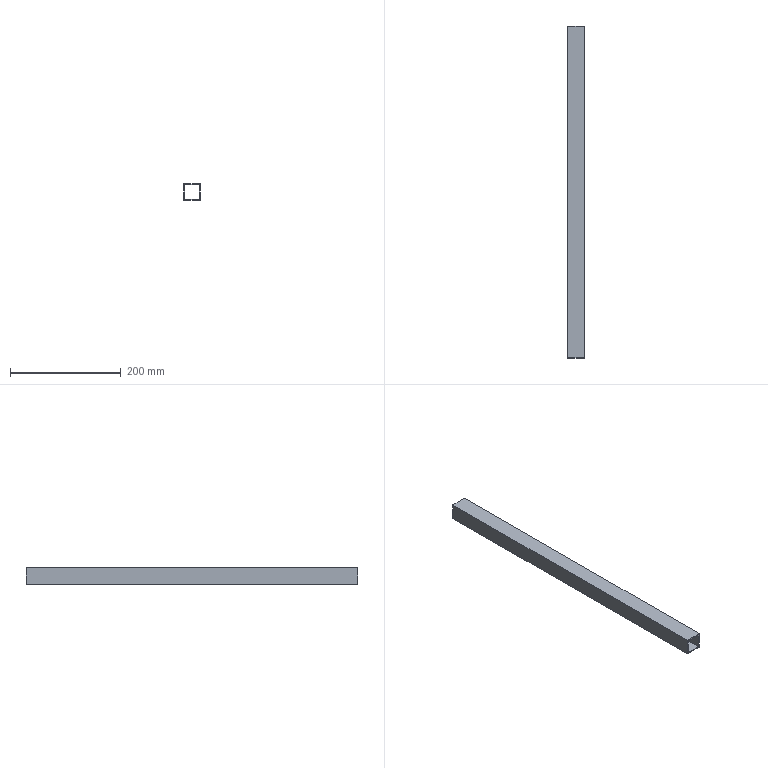Part | NX | features solid 2 | 1 solid | 10 faces | box 30 x 600 x 30 mm | volume 134400 mm3 | plane 10
STEP:
#1=CARTESIAN_POINT('',(-135.,-330.,-30.));
#2=VERTEX_POINT('',#1);
#3=CARTESIAN_POINT('',(-105.,-330.,-30.));
#4=VERTEX_POINT('',#3);
#5=CARTESIAN_POINT('',(-320.,-330.,-30.));
#6=DIRECTION('',(1.,0.,0.));
#7=VECTOR('',#6,1000.);
#8=LINE('',#5,#7);
#9=EDGE_CURVE('',#2,#4,#8,.T.);
#10=ORIENTED_EDGE('',*,*,#9,.T.);
#11=CARTESIAN_POINT('',(-105.,-330.,0.));
#12=VERTEX_POINT('',#11);
#13=CARTESIAN_POINT('',(-105.,-330.,0.));
#14=DIRECTION('',(0.,0.,-1.));
#15=VECTOR('',#14,1000.);
#16=LINE('',#13,#15);
#17=EDGE_CURVE('',#12,#4,#16,.T.);
#18=ORIENTED_EDGE('',*,*,#17,.F.);
#19=CARTESIAN_POINT('',(-135.,-330.,0.));
#20=VERTEX_POINT('',#19);
#21=CARTESIAN_POINT('',(-320.,-330.,0.));
#22=DIRECTION('',(1.,0.,0.));
#23=VECTOR('',#22,1000.);
#24=LINE('',#21,#23);
#25=EDGE_CURVE('',#20,#12,#24,.T.);
#26=ORIENTED_EDGE('',*,*,#25,.F.);
#27=CARTESIAN_POINT('',(-135.,-330.,0.));
#28=DIRECTION('',(0.,0.,-1.));
#29=VECTOR('',#28,1000.);
#30=LINE('',#27,#29);
#31=EDGE_CURVE('',#20,#2,#30,.T.);
#32=ORIENTED_EDGE('',*,*,#31,.T.);
#33=EDGE_LOOP('',(#10,#18,#26,#32));
#34=FACE_BOUND('',#33,.T.);
#35=CARTESIAN_POINT('',(-133.,-330.,-28.));
#36=VERTEX_POINT('',#35);
#37=CARTESIAN_POINT('',(-107.,-330.,-28.));
#38=VERTEX_POINT('',#37);
#39=CARTESIAN_POINT('',(-320.,-330.,-28.));
#40=DIRECTION('',(1.,0.,0.));
#41=VECTOR('',#40,1000.);
#42=LINE('',#39,#41);
#43=EDGE_CURVE('',#36,#38,#42,.T.);
#44=ORIENTED_EDGE('',*,*,#43,.F.);
#45=CARTESIAN_POINT('',(-133.,-330.,-2.));
#46=VERTEX_POINT('',#45);
#47=CARTESIAN_POINT('',(-133.,-330.,0.));
#48=DIRECTION('',(0.,0.,-1.));
#49=VECTOR('',#48,1000.);
#50=LINE('',#47,#49);
#51=EDGE_CURVE('',#46,#36,#50,.T.);
#52=ORIENTED_EDGE('',*,*,#51,.F.);
#53=CARTESIAN_POINT('',(-107.,-330.,-2.));
#54=VERTEX_POINT('',#53);
#55=CARTESIAN_POINT('',(-320.,-330.,-2.));
#56=DIRECTION('',(1.,0.,0.));
#57=VECTOR('',#56,1000.);
#58=LINE('',#55,#57);
#59=EDGE_CURVE('',#46,#54,#58,.T.);
#60=ORIENTED_EDGE('',*,*,#59,.T.);
#61=CARTESIAN_POINT('',(-107.,-330.,0.));
#62=DIRECTION('',(0.,0.,-1.));
#63=VECTOR('',#62,1000.);
#64=LINE('',#61,#63);
#65=EDGE_CURVE('',#54,#38,#64,.T.);
#66=ORIENTED_EDGE('',*,*,#65,.T.);
#67=EDGE_LOOP('',(#44,#52,#60,#66));
#68=FACE_BOUND('',#67,.T.);
#69=CARTESIAN_POINT('',(-320.,-330.,0.));
#70=DIRECTION('',(0.,1.,0.));
#71=DIRECTION('',(0.,0.,1.));
#72=AXIS2_PLACEMENT_3D('',#69,#70,#71);
#73=PLANE('',#72);
#74=ADVANCED_FACE('',(#34,#68),#73,.F.);
#75=CARTESIAN_POINT('',(-135.,270.,0.));
#76=VERTEX_POINT('',#75);
#77=CARTESIAN_POINT('',(-135.,-330.,0.));
#78=DIRECTION('',(0.,1.,0.));
#79=VECTOR('',#78,1000.);
#80=LINE('',#77,#79);
#81=EDGE_CURVE('',#20,#76,#80,.T.);
#82=ORIENTED_EDGE('',*,*,#81,.T.);
#83=CARTESIAN_POINT('',(-135.,270.,-30.));
#84=VERTEX_POINT('',#83);
#85=CARTESIAN_POINT('',(-135.,270.,0.));
#86=DIRECTION('',(0.,0.,1.));
#87=VECTOR('',#86,1000.);
#88=LINE('',#85,#87);
#89=EDGE_CURVE('',#84,#76,#88,.T.);
#90=ORIENTED_EDGE('',*,*,#89,.F.);
#91=CARTESIAN_POINT('',(-135.,-330.,-30.));
#92=DIRECTION('',(0.,1.,0.));
#93=VECTOR('',#92,1000.);
#94=LINE('',#91,#93);
#95=EDGE_CURVE('',#2,#84,#94,.T.);
#96=ORIENTED_EDGE('',*,*,#95,.F.);
#97=ORIENTED_EDGE('',*,*,#31,.F.);
#98=EDGE_LOOP('',(#82,#90,#96,#97));
#99=FACE_BOUND('',#98,.T.);
#100=CARTESIAN_POINT('',(-135.,-330.,0.));
#101=DIRECTION('',(-1.,0.,0.));
#102=DIRECTION('',(0.,0.,1.));
#103=AXIS2_PLACEMENT_3D('',#100,#101,#102);
#104=PLANE('',#103);
#105=ADVANCED_FACE('',(#99),#104,.T.);
#106=CARTESIAN_POINT('',(-105.,270.,-30.));
#107=VERTEX_POINT('',#106);
#108=CARTESIAN_POINT('',(-105.,-330.,-30.));
#109=DIRECTION('',(0.,1.,0.));
#110=VECTOR('',#109,1000.);
#111=LINE('',#108,#110);
#112=EDGE_CURVE('',#4,#107,#111,.T.);
#113=ORIENTED_EDGE('',*,*,#112,.T.);
#114=CARTESIAN_POINT('',(-105.,270.,0.));
#115=VERTEX_POINT('',#114);
#116=CARTESIAN_POINT('',(-105.,270.,0.));
#117=DIRECTION('',(0.,0.,1.));
#118=VECTOR('',#117,1000.);
#119=LINE('',#116,#118);
#120=EDGE_CURVE('',#107,#115,#119,.T.);
#121=ORIENTED_EDGE('',*,*,#120,.T.);
#122=CARTESIAN_POINT('',(-105.,-330.,0.));
#123=DIRECTION('',(0.,1.,0.));
#124=VECTOR('',#123,1000.);
#125=LINE('',#122,#124);
#126=EDGE_CURVE('',#12,#115,#125,.T.);
#127=ORIENTED_EDGE('',*,*,#126,.F.);
#128=ORIENTED_EDGE('',*,*,#17,.T.);
#129=EDGE_LOOP('',(#113,#121,#127,#128));
#130=FACE_BOUND('',#129,.T.);
#131=CARTESIAN_POINT('',(-105.,-330.,0.));
#132=DIRECTION('',(-1.,0.,0.));
#133=DIRECTION('',(0.,0.,1.));
#134=AXIS2_PLACEMENT_3D('',#131,#132,#133);
#135=PLANE('',#134);
#136=ADVANCED_FACE('',(#130),#135,.F.);
#137=ORIENTED_EDGE('',*,*,#126,.T.);
#138=CARTESIAN_POINT('',(-248.75,270.,0.));
#139=DIRECTION('',(1.,0.,0.));
#140=VECTOR('',#139,1000.);
#141=LINE('',#138,#140);
#142=EDGE_CURVE('',#76,#115,#141,.T.);
#143=ORIENTED_EDGE('',*,*,#142,.F.);
#144=ORIENTED_EDGE('',*,*,#81,.F.);
#145=ORIENTED_EDGE('',*,*,#25,.T.);
#146=EDGE_LOOP('',(#137,#143,#144,#145));
#147=FACE_BOUND('',#146,.T.);
#148=CARTESIAN_POINT('',(-248.75,-180.,0.));
#149=DIRECTION('',(0.,0.,1.));
#150=DIRECTION('',(1.,0.,0.));
#151=AXIS2_PLACEMENT_3D('',#148,#149,#150);
#152=PLANE('',#151);
#153=ADVANCED_FACE('',(#147),#152,.T.);
#154=ORIENTED_EDGE('',*,*,#95,.T.);
#155=CARTESIAN_POINT('',(-248.75,270.,-30.));
#156=DIRECTION('',(1.,0.,0.));
#157=VECTOR('',#156,1000.);
#158=LINE('',#155,#157);
#159=EDGE_CURVE('',#84,#107,#158,.T.);
#160=ORIENTED_EDGE('',*,*,#159,.T.);
#161=ORIENTED_EDGE('',*,*,#112,.F.);
#162=ORIENTED_EDGE('',*,*,#9,.F.);
#163=EDGE_LOOP('',(#154,#160,#161,#162));
#164=FACE_BOUND('',#163,.T.);
#165=CARTESIAN_POINT('',(-248.75,-180.,-30.));
#166=DIRECTION('',(0.,0.,1.));
#167=DIRECTION('',(1.,0.,0.));
#168=AXIS2_PLACEMENT_3D('',#165,#166,#167);
#169=PLANE('',#168);
#170=ADVANCED_FACE('',(#164),#169,.F.);
#171=CARTESIAN_POINT('',(-133.,270.,-28.));
#172=VERTEX_POINT('',#171);
#173=CARTESIAN_POINT('',(-133.,-330.,-28.));
#174=DIRECTION('',(0.,1.,0.));
#175=VECTOR('',#174,1000.);
#176=LINE('',#173,#175);
#177=EDGE_CURVE('',#36,#172,#176,.T.);
#178=ORIENTED_EDGE('',*,*,#177,.T.);
#179=CARTESIAN_POINT('',(-133.,270.,-2.));
#180=VERTEX_POINT('',#179);
#181=CARTESIAN_POINT('',(-133.,270.,0.));
#182=DIRECTION('',(0.,0.,1.));
#183=VECTOR('',#182,1000.);
#184=LINE('',#181,#183);
#185=EDGE_CURVE('',#172,#180,#184,.T.);
#186=ORIENTED_EDGE('',*,*,#185,.T.);
#187=CARTESIAN_POINT('',(-133.,-330.,-2.));
#188=DIRECTION('',(0.,1.,0.));
#189=VECTOR('',#188,1000.);
#190=LINE('',#187,#189);
#191=EDGE_CURVE('',#46,#180,#190,.T.);
#192=ORIENTED_EDGE('',*,*,#191,.F.);
#193=ORIENTED_EDGE('',*,*,#51,.T.);
#194=EDGE_LOOP('',(#178,#186,#192,#193));
#195=FACE_BOUND('',#194,.T.);
#196=CARTESIAN_POINT('',(-133.,-330.,0.));
#197=DIRECTION('',(-1.,0.,0.));
#198=DIRECTION('',(0.,0.,1.));
#199=AXIS2_PLACEMENT_3D('',#196,#197,#198);
#200=PLANE('',#199);
#201=ADVANCED_FACE('',(#195),#200,.F.);
#202=CARTESIAN_POINT('',(-107.,270.,-2.));
#203=VERTEX_POINT('',#202);
#204=CARTESIAN_POINT('',(-107.,-330.,-2.));
#205=DIRECTION('',(0.,1.,0.));
#206=VECTOR('',#205,1000.);
#207=LINE('',#204,#206);
#208=EDGE_CURVE('',#54,#203,#207,.T.);
#209=ORIENTED_EDGE('',*,*,#208,.T.);
#210=CARTESIAN_POINT('',(-107.,270.,-28.));
#211=VERTEX_POINT('',#210);
#212=CARTESIAN_POINT('',(-107.,270.,0.));
#213=DIRECTION('',(0.,0.,1.));
#214=VECTOR('',#213,1000.);
#215=LINE('',#212,#214);
#216=EDGE_CURVE('',#211,#203,#215,.T.);
#217=ORIENTED_EDGE('',*,*,#216,.F.);
#218=CARTESIAN_POINT('',(-107.,-330.,-28.));
#219=DIRECTION('',(0.,1.,0.));
#220=VECTOR('',#219,1000.);
#221=LINE('',#218,#220);
#222=EDGE_CURVE('',#38,#211,#221,.T.);
#223=ORIENTED_EDGE('',*,*,#222,.F.);
#224=ORIENTED_EDGE('',*,*,#65,.F.);
#225=EDGE_LOOP('',(#209,#217,#223,#224));
#226=FACE_BOUND('',#225,.T.);
#227=CARTESIAN_POINT('',(-107.,-330.,0.));
#228=DIRECTION('',(-1.,0.,0.));
#229=DIRECTION('',(0.,0.,1.));
#230=AXIS2_PLACEMENT_3D('',#227,#228,#229);
#231=PLANE('',#230);
#232=ADVANCED_FACE('',(#226),#231,.T.);
#233=ORIENTED_EDGE('',*,*,#191,.T.);
#234=CARTESIAN_POINT('',(-248.75,270.,-2.));
#235=DIRECTION('',(1.,0.,0.));
#236=VECTOR('',#235,1000.);
#237=LINE('',#234,#236);
#238=EDGE_CURVE('',#180,#203,#237,.T.);
#239=ORIENTED_EDGE('',*,*,#238,.T.);
#240=ORIENTED_EDGE('',*,*,#208,.F.);
#241=ORIENTED_EDGE('',*,*,#59,.F.);
#242=EDGE_LOOP('',(#233,#239,#240,#241));
#243=FACE_BOUND('',#242,.T.);
#244=CARTESIAN_POINT('',(-248.75,-180.,-2.));
#245=DIRECTION('',(0.,0.,1.));
#246=DIRECTION('',(1.,0.,0.));
#247=AXIS2_PLACEMENT_3D('',#244,#245,#246);
#248=PLANE('',#247);
#249=ADVANCED_FACE('',(#243),#248,.F.);
#250=ORIENTED_EDGE('',*,*,#222,.T.);
#251=CARTESIAN_POINT('',(-248.75,270.,-28.));
#252=DIRECTION('',(1.,0.,0.));
#253=VECTOR('',#252,1000.);
#254=LINE('',#251,#253);
#255=EDGE_CURVE('',#172,#211,#254,.T.);
#256=ORIENTED_EDGE('',*,*,#255,.F.);
#257=ORIENTED_EDGE('',*,*,#177,.F.);
#258=ORIENTED_EDGE('',*,*,#43,.T.);
#259=EDGE_LOOP('',(#250,#256,#257,#258));
#260=FACE_BOUND('',#259,.T.);
#261=CARTESIAN_POINT('',(-248.75,-180.,-28.));
#262=DIRECTION('',(0.,0.,1.));
#263=DIRECTION('',(1.,0.,0.));
#264=AXIS2_PLACEMENT_3D('',#261,#262,#263);
#265=PLANE('',#264);
#266=ADVANCED_FACE('',(#260),#265,.T.);
#267=ORIENTED_EDGE('',*,*,#142,.T.);
#268=ORIENTED_EDGE('',*,*,#120,.F.);
#269=ORIENTED_EDGE('',*,*,#159,.F.);
#270=ORIENTED_EDGE('',*,*,#89,.T.);
#271=EDGE_LOOP('',(#267,#268,#269,#270));
#272=FACE_BOUND('',#271,.T.);
#273=ORIENTED_EDGE('',*,*,#185,.F.);
#274=ORIENTED_EDGE('',*,*,#255,.T.);
#275=ORIENTED_EDGE('',*,*,#216,.T.);
#276=ORIENTED_EDGE('',*,*,#238,.F.);
#277=EDGE_LOOP('',(#273,#274,#275,#276));
#278=FACE_BOUND('',#277,.T.);
#279=CARTESIAN_POINT('',(0.,270.,-115.));
#280=DIRECTION('',(0.,-1.,0.));
#281=DIRECTION('',(0.,0.,-1.));
#282=AXIS2_PLACEMENT_3D('',#279,#280,#281);
#283=PLANE('',#282);
#284=ADVANCED_FACE('',(#272,#278),#283,.F.);
#285=CLOSED_SHELL('',(#74,#105,#136,#153,#170,#201,#232,#249,#266,#284));
#286=MANIFOLD_SOLID_BREP('',#285);
#287=(LENGTH_UNIT()NAMED_UNIT(*)SI_UNIT(.MILLI.,.METRE.));
#288=UNCERTAINTY_MEASURE_WITH_UNIT(LENGTH_MEASURE(0.00001),#287,'','');
#289=(NAMED_UNIT(*)PLANE_ANGLE_UNIT()SI_UNIT($,.RADIAN.));
#290=(NAMED_UNIT(*)SI_UNIT($,.STERADIAN.)SOLID_ANGLE_UNIT());
#291=(GEOMETRIC_REPRESENTATION_CONTEXT(3)GLOBAL_UNCERTAINTY_ASSIGNED_CONTEXT((#288))GLOBAL_UNIT_ASSIGNED_CONTEXT((#287,#289,#290))REPRESENTATION_CONTEXT('',''));
#292=ADVANCED_BREP_SHAPE_REPRESENTATION('',(#286),#291);